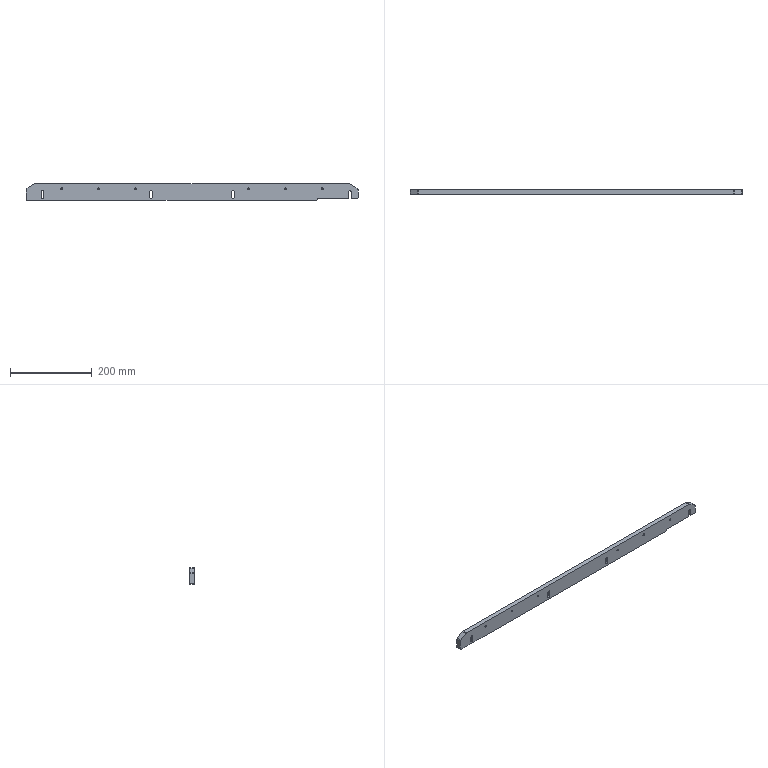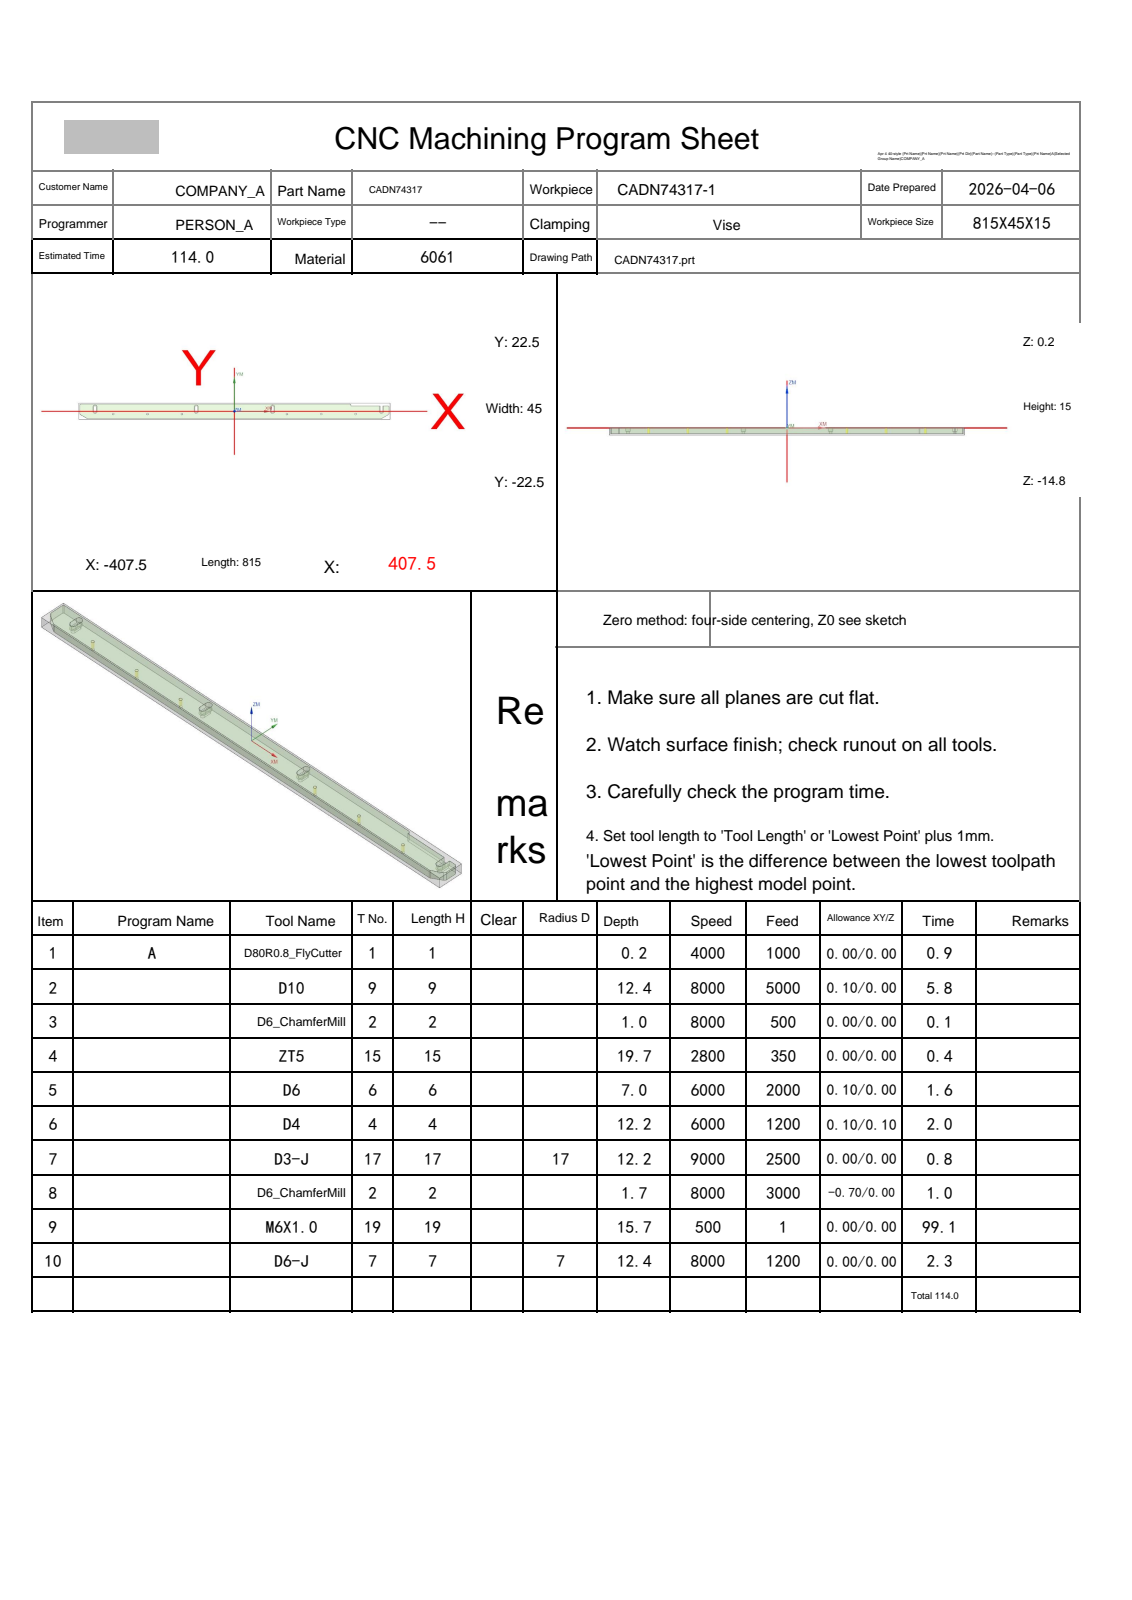NC program | NX | posted by the shop | part box 810 x 12 x 40 mm
Lines 1 to 1438 of 3610, first 1187 of 1436 lines:
%
O0001
(Machine time: 209.16 MIN)
(===Total Tool:9===)
(T1=D80R0.8 FlyCutter D=80.  R=0.8  D-  H01 Z=-0.   )
(T9=D10     D=10.  R=0.   D-  H09 Z=-12.2 )
(T2=D6_ChamferMill   D=6.   R=0.   D-  H02 Z=-1.5  )
(T15=ZT5    D=5.   DR_a=118 D-  H15 Z=-19.5 )
(T6=D6      D=6.   R=0.   D-  H06 Z=-6.8  )
(T4=D4      D=4.   R=0.   D-  H04 Z=-12.  )
(T17=D3-J   D=3.   R=0.   D17 H17 Z=-12.  )
(T19=M6X1.0 D=5.   DR_a=180 D-  H19 Z=-15.5 )
(T7=D6-J    D=6.   R=0.   D7  H07 Z=-12.2 )
G80 G90 G17 G49 G40
G91 G28 Z0
M01
N1 T01 M06
(D80R0.8 FlyCutter  D=80. R=0.8 H=01 ce=0.00 di=0.00)
G00 G90 G54 X450. Y0.0 M03 S4000
G43 H01 Z20.
M08
Z2.
G01 Z0.0 F1000.
X445.
X-445.
X-450.
Z2.
G00 Z20.
G91 G28 Z0.0
M05
M09
G91 G28 Z0.0
M01
N2 T09 M06
(D10  D=10. R=0. H=09 ce=0.10 di=0.00)
G00 G90 G54 X0.0 Y-25.1 M03 S8000
G43 H09 Z20.
M08
Z.5
G01 X-383.615 Z.322 F5000.
G02 X-388.811 Y-23.661 Z.319 I0.0 J10.1
G01 X-405.196 Y-13.83 Z.31
G02 X-410.1 Y-5.169 Z.306 I5.196 J8.661
G01 Y18. Z.295
G02 X-408.606 Y21.606 Z.293 I5.1 J0.0
G01 X-406.606 Y23.606 Z.292
G02 X-403. Y25.1 Z.29 I3.606 J-3.606
G01 X303. Z-.038
G02 X306.606 Y23.606 Z-.04 I0.0 J-5.1
G01 X308.606 Y21.606 Z-.041
G02 X309.648 Y20.1 Z-.042 I-3.606 J-3.606
G01 X381.7 Z-.076
G02 X385. Y18.888 Z-.077 I0.0 J-5.1
X388.3 Y20.1 Z-.079 I3.3 J-3.888
G01 X403. Z-.086
G02 X406.606 Y18.606 Z-.088 I0.0 J-5.1
G01 X408.606 Y16.606 Z-.089
G02 X410.1 Y13. Z-.091 I-3.606 J-3.606
G01 Y-5.169 Z-.099
G02 X405.196 Y-13.83 Z-.104 I-10.1 J0.0
G01 X388.811 Y-23.661 Z-.113
G02 X383.615 Y-25.1 Z-.116 I-5.196 J8.661
G01 X-383.615 Z-.472
G02 X-388.811 Y-23.661 Z-.474 I0.0 J10.1
G01 X-405.196 Y-13.83 Z-.483
G02 X-410.1 Y-5.169 Z-.488 I5.196 J8.661
G01 Y18. Z-.499
G02 X-408.606 Y21.606 Z-.501 I5.1 J0.0
G01 X-406.606 Y23.606 Z-.502
G02 X-403. Y25.1 Z-.504 I3.606 J-3.606
G01 X303. Z-.832
G02 X306.606 Y23.606 Z-.834 I0.0 J-5.1
G01 X308.606 Y21.606 Z-.835
G02 X309.648 Y20.1 Z-.836 I-3.606 J-3.606
G01 X381.7 Z-.869
G02 X385. Y18.888 Z-.871 I0.0 J-5.1
X388.3 Y20.1 Z-.873 I3.3 J-3.888
G01 X403. Z-.88
G02 X406.606 Y18.606 Z-.881 I0.0 J-5.1
G01 X408.606 Y16.606 Z-.883
G02 X410.1 Y13. Z-.885 I-3.606 J-3.606
G01 Y-5.169 Z-.893
G02 X405.196 Y-13.83 Z-.898 I-10.1 J0.0
G01 X388.811 Y-23.661 Z-.907
G02 X383.615 Y-25.1 Z-.909 I-5.196 J8.661
G01 X-383.615 Z-1.266
G02 X-388.811 Y-23.661 Z-1.268 I0.0 J10.1
G01 X-405.196 Y-13.83 Z-1.277
G02 X-410.1 Y-5.169 Z-1.282 I5.196 J8.661
G01 Y18. Z-1.293
G02 X-408.606 Y21.606 Z-1.295 I5.1 J0.0
G01 X-406.606 Y23.606 Z-1.296
G02 X-403. Y25.1 Z-1.298 I3.606 J-3.606
G01 X303. Z-1.626
G02 X306.606 Y23.606 Z-1.628 I0.0 J-5.1
G01 X308.606 Y21.606 Z-1.629
G02 X309.648 Y20.1 Z-1.63 I-3.606 J-3.606
G01 X381.7 Z-1.663
G02 X385. Y18.888 Z-1.665 I0.0 J-5.1
X388.3 Y20.1 Z-1.667 I3.3 J-3.888
G01 X403. Z-1.673
G02 X406.606 Y18.606 Z-1.675 I0.0 J-5.1
G01 X408.606 Y16.606 Z-1.677
G02 X410.1 Y13. Z-1.678 I-3.606 J-3.606
G01 Y-5.169 Z-1.687
G02 X405.196 Y-13.83 Z-1.692 I-10.1 J0.0
G01 X388.811 Y-23.661 Z-1.701
G02 X383.615 Y-25.1 Z-1.703 I-5.196 J8.661
G01 X-383.615 Z-2.059
G02 X-388.811 Y-23.661 Z-2.062 I0.0 J10.1
G01 X-405.196 Y-13.83 Z-2.071
G02 X-410.1 Y-5.169 Z-2.076 I5.196 J8.661
G01 Y18. Z-2.086
G02 X-408.606 Y21.606 Z-2.088 I5.1 J0.0
G01 X-406.606 Y23.606 Z-2.09
G02 X-403. Y25.1 Z-2.091 I3.606 J-3.606
G01 X303. Z-2.419
G02 X306.606 Y23.606 Z-2.421 I0.0 J-5.1
G01 X308.606 Y21.606 Z-2.423
G02 X309.648 Y20.1 Z-2.423 I-3.606 J-3.606
G01 X381.7 Z-2.457
G02 X385. Y18.888 Z-2.459 I0.0 J-5.1
X388.3 Y20.1 Z-2.46 I3.3 J-3.888
G01 X403. Z-2.467
G02 X406.606 Y18.606 Z-2.469 I0.0 J-5.1
G01 X408.606 Y16.606 Z-2.47
G02 X410.1 Y13. Z-2.472 I-3.606 J-3.606
G01 Y-5.169 Z-2.481
G02 X405.196 Y-13.83 Z-2.485 I-10.1 J0.0
G01 X388.811 Y-23.661 Z-2.494
G02 X383.615 Y-25.1 Z-2.497 I-5.196 J8.661
G01 X-383.615 Z-2.853
G02 X-388.811 Y-23.661 Z-2.856 I0.0 J10.1
G01 X-405.196 Y-13.83 Z-2.865
G02 X-410.1 Y-5.169 Z-2.869 I5.196 J8.661
G01 Y18. Z-2.88
G02 X-408.606 Y21.606 Z-2.882 I5.1 J0.0
G01 X-406.606 Y23.606 Z-2.883
G02 X-403. Y25.1 Z-2.885 I3.606 J-3.606
G01 X303. Z-3.213
G02 X306.606 Y23.606 Z-3.215 I0.0 J-5.1
G01 X308.606 Y21.606 Z-3.216
G02 X309.648 Y20.1 Z-3.217 I-3.606 J-3.606
G01 X381.7 Z-3.251
G02 X385. Y18.888 Z-3.252 I0.0 J-5.1
X388.3 Y20.1 Z-3.254 I3.3 J-3.888
G01 X403. Z-3.261
G02 X406.606 Y18.606 Z-3.263 I0.0 J-5.1
G01 X408.606 Y16.606 Z-3.264
G02 X410.1 Y13. Z-3.266 I-3.606 J-3.606
G01 Y-5.169 Z-3.274
G02 X405.196 Y-13.83 Z-3.279 I-10.1 J0.0
G01 X388.811 Y-23.661 Z-3.288
G02 X383.615 Y-25.1 Z-3.291 I-5.196 J8.661
G01 X-383.615 Z-3.647
G02 X-388.811 Y-23.661 Z-3.649 I0.0 J10.1
G01 X-405.196 Y-13.83 Z-3.658
G02 X-410.1 Y-5.169 Z-3.663 I5.196 J8.661
G01 Y18. Z-3.674
G02 X-408.606 Y21.606 Z-3.676 I5.1 J0.0
G01 X-406.606 Y23.606 Z-3.677
G02 X-403. Y25.1 Z-3.679 I3.606 J-3.606
G01 X303. Z-4.007
G02 X306.606 Y23.606 Z-4.009 I0.0 J-5.1
G01 X308.606 Y21.606 Z-4.01
G02 X309.648 Y20.1 Z-4.011 I-3.606 J-3.606
G01 X381.7 Z-4.044
G02 X385. Y18.888 Z-4.046 I0.0 J-5.1
X388.3 Y20.1 Z-4.048 I3.3 J-3.888
G01 X403. Z-4.055
G02 X406.606 Y18.606 Z-4.056 I0.0 J-5.1
G01 X408.606 Y16.606 Z-4.058
G02 X410.1 Y13. Z-4.06 I-3.606 J-3.606
G01 Y-5.169 Z-4.068
G02 X405.196 Y-13.83 Z-4.073 I-10.1 J0.0
G01 X388.811 Y-23.661 Z-4.082
G02 X383.615 Y-25.1 Z-4.084 I-5.196 J8.661
G01 X-383.615 Z-4.441
G02 X-388.811 Y-23.661 Z-4.443 I0.0 J10.1
G01 X-405.196 Y-13.83 Z-4.452
G02 X-410.1 Y-5.169 Z-4.457 I5.196 J8.661
G01 Y18. Z-4.468
G02 X-408.606 Y21.606 Z-4.47 I5.1 J0.0
G01 X-406.606 Y23.606 Z-4.471
G02 X-403. Y25.1 Z-4.473 I3.606 J-3.606
G01 X303. Z-4.801
G02 X306.606 Y23.606 Z-4.803 I0.0 J-5.1
G01 X308.606 Y21.606 Z-4.804
G02 X309.648 Y20.1 Z-4.805 I-3.606 J-3.606
G01 X381.7 Z-4.838
G02 X385. Y18.888 Z-4.84 I0.0 J-5.1
X388.3 Y20.1 Z-4.842 I3.3 J-3.888
G01 X403. Z-4.848
G02 X406.606 Y18.606 Z-4.85 I0.0 J-5.1
G01 X408.606 Y16.606 Z-4.852
G02 X410.1 Y13. Z-4.853 I-3.606 J-3.606
G01 Y-5.169 Z-4.862
G02 X405.196 Y-13.83 Z-4.867 I-10.1 J0.0
G01 X388.811 Y-23.661 Z-4.876
G02 X383.615 Y-25.1 Z-4.878 I-5.196 J8.661
G01 X-383.615 Z-5.234
G02 X-388.811 Y-23.661 Z-5.237 I0.0 J10.1
G01 X-405.196 Y-13.83 Z-5.246
G02 X-410.1 Y-5.169 Z-5.251 I5.196 J8.661
G01 Y18. Z-5.261
G02 X-408.606 Y21.606 Z-5.263 I5.1 J0.0
G01 X-406.606 Y23.606 Z-5.265
G02 X-403. Y25.1 Z-5.266 I3.606 J-3.606
G01 X303. Z-5.594
G02 X306.606 Y23.606 Z-5.596 I0.0 J-5.1
G01 X308.606 Y21.606 Z-5.598
G02 X309.648 Y20.1 Z-5.598 I-3.606 J-3.606
G01 X381.7 Z-5.632
G02 X385. Y18.888 Z-5.634 I0.0 J-5.1
X388.3 Y20.1 Z-5.635 I3.3 J-3.888
G01 X403. Z-5.642
G02 X406.606 Y18.606 Z-5.644 I0.0 J-5.1
G01 X408.606 Y16.606 Z-5.645
G02 X410.1 Y13. Z-5.647 I-3.606 J-3.606
G01 Y-5.169 Z-5.656
G02 X405.196 Y-13.83 Z-5.66 I-10.1 J0.0
G01 X388.811 Y-23.661 Z-5.669
G02 X383.615 Y-25.1 Z-5.672 I-5.196 J8.661
G01 X-383.615 Z-6.028
G02 X-388.811 Y-23.661 Z-6.031 I0.0 J10.1
G01 X-405.196 Y-13.83 Z-6.04
G02 X-410.1 Y-5.169 Z-6.044 I5.196 J8.661
G01 Y18. Z-6.055
G02 X-408.606 Y21.606 Z-6.057 I5.1 J0.0
G01 X-406.606 Y23.606 Z-6.058
G02 X-403. Y25.1 Z-6.06 I3.606 J-3.606
G01 X303. Z-6.388
G02 X306.606 Y23.606 Z-6.39 I0.0 J-5.1
G01 X308.606 Y21.606 Z-6.391
G02 X309.648 Y20.1 Z-6.392 I-3.606 J-3.606
G01 X381.7 Z-6.426
G02 X385. Y18.888 Z-6.427 I0.0 J-5.1
X388.3 Y20.1 Z-6.429 I3.3 J-3.888
G01 X403. Z-6.436
G02 X406.606 Y18.606 Z-6.438 I0.0 J-5.1
G01 X408.606 Y16.606 Z-6.439
G02 X410.1 Y13. Z-6.441 I-3.606 J-3.606
G01 Y-5.169 Z-6.449
G02 X405.196 Y-13.83 Z-6.454 I-10.1 J0.0
G01 X388.811 Y-23.661 Z-6.463
G02 X383.615 Y-25.1 Z-6.466 I-5.196 J8.661
G01 X-383.615 Z-6.822
G02 X-388.811 Y-23.661 Z-6.824 I0.0 J10.1
G01 X-405.196 Y-13.83 Z-6.833
G02 X-410.1 Y-5.169 Z-6.838 I5.196 J8.661
G01 Y18. Z-6.849
G02 X-408.606 Y21.606 Z-6.851 I5.1 J0.0
G01 X-406.606 Y23.606 Z-6.852
G02 X-403. Y25.1 Z-6.854 I3.606 J-3.606
G01 X303. Z-7.182
G02 X306.606 Y23.606 Z-7.184 I0.0 J-5.1
G01 X308.606 Y21.606 Z-7.185
G02 X309.648 Y20.1 Z-7.186 I-3.606 J-3.606
G01 X381.7 Z-7.219
G02 X385. Y18.888 Z-7.221 I0.0 J-5.1
X388.3 Y20.1 Z-7.223 I3.3 J-3.888
G01 X403. Z-7.23
G02 X406.606 Y18.606 Z-7.231 I0.0 J-5.1
G01 X408.606 Y16.606 Z-7.233
G02 X410.1 Y13. Z-7.235 I-3.606 J-3.606
G01 Y-5.169 Z-7.243
G02 X405.196 Y-13.83 Z-7.248 I-10.1 J0.0
G01 X388.811 Y-23.661 Z-7.257
G02 X383.615 Y-25.1 Z-7.259 I-5.196 J8.661
G01 X-383.615 Z-7.616
G02 X-388.811 Y-23.661 Z-7.618 I0.0 J10.1
G01 X-405.196 Y-13.83 Z-7.627
G02 X-410.1 Y-5.169 Z-7.632 I5.196 J8.661
G01 Y18. Z-7.643
G02 X-408.606 Y21.606 Z-7.645 I5.1 J0.0
G01 X-406.606 Y23.606 Z-7.646
G02 X-403. Y25.1 Z-7.648 I3.606 J-3.606
G01 X303. Z-7.976
G02 X306.606 Y23.606 Z-7.978 I0.0 J-5.1
G01 X308.606 Y21.606 Z-7.979
G02 X309.648 Y20.1 Z-7.98 I-3.606 J-3.606
G01 X381.7 Z-8.013
G02 X385. Y18.888 Z-8.015 I0.0 J-5.1
X388.3 Y20.1 Z-8.017 I3.3 J-3.888
G01 X403. Z-8.023
G02 X406.606 Y18.606 Z-8.025 I0.0 J-5.1
G01 X408.606 Y16.606 Z-8.027
G02 X410.1 Y13. Z-8.028 I-3.606 J-3.606
G01 Y-5.169 Z-8.037
G02 X405.196 Y-13.83 Z-8.042 I-10.1 J0.0
G01 X388.811 Y-23.661 Z-8.051
G02 X383.615 Y-25.1 Z-8.053 I-5.196 J8.661
G01 X-383.615 Z-8.409
G02 X-388.811 Y-23.661 Z-8.412 I0.0 J10.1
G01 X-405.196 Y-13.83 Z-8.421
G02 X-410.1 Y-5.169 Z-8.426 I5.196 J8.661
G01 Y18. Z-8.436
G02 X-408.606 Y21.606 Z-8.438 I5.1 J0.0
G01 X-406.606 Y23.606 Z-8.44
G02 X-403. Y25.1 Z-8.441 I3.606 J-3.606
G01 X303. Z-8.769
G02 X306.606 Y23.606 Z-8.771 I0.0 J-5.1
G01 X308.606 Y21.606 Z-8.773
G02 X309.648 Y20.1 Z-8.773 I-3.606 J-3.606
G01 X381.7 Z-8.807
G02 X385. Y18.888 Z-8.809 I0.0 J-5.1
X388.3 Y20.1 Z-8.81 I3.3 J-3.888
G01 X403. Z-8.817
G02 X406.606 Y18.606 Z-8.819 I0.0 J-5.1
G01 X408.606 Y16.606 Z-8.82
G02 X410.1 Y13. Z-8.822 I-3.606 J-3.606
G01 Y-5.169 Z-8.831
G02 X405.196 Y-13.83 Z-8.835 I-10.1 J0.0
G01 X388.811 Y-23.661 Z-8.844
G02 X383.615 Y-25.1 Z-8.847 I-5.196 J8.661
G01 X-383.615 Z-9.203
G02 X-388.811 Y-23.661 Z-9.206 I0.0 J10.1
G01 X-405.196 Y-13.83 Z-9.215
G02 X-410.1 Y-5.169 Z-9.219 I5.196 J8.661
G01 Y18. Z-9.23
G02 X-408.606 Y21.606 Z-9.232 I5.1 J0.0
G01 X-406.606 Y23.606 Z-9.233
G02 X-403. Y25.1 Z-9.235 I3.606 J-3.606
G01 X303. Z-9.563
G02 X306.606 Y23.606 Z-9.565 I0.0 J-5.1
G01 X308.606 Y21.606 Z-9.566
G02 X309.648 Y20.1 Z-9.567 I-3.606 J-3.606
G01 X381.7 Z-9.601
G02 X385. Y18.888 Z-9.602 I0.0 J-5.1
X388.3 Y20.1 Z-9.604 I3.3 J-3.888
G01 X403. Z-9.611
G02 X406.606 Y18.606 Z-9.613 I0.0 J-5.1
G01 X408.606 Y16.606 Z-9.614
G02 X410.1 Y13. Z-9.616 I-3.606 J-3.606
G01 Y-5.169 Z-9.624
G02 X405.196 Y-13.83 Z-9.629 I-10.1 J0.0
G01 X388.811 Y-23.661 Z-9.638
G02 X383.615 Y-25.1 Z-9.641 I-5.196 J8.661
G01 X-383.615 Z-9.997
G02 X-388.811 Y-23.661 Z-9.999 I0.0 J10.1
G01 X-405.196 Y-13.83 Z-10.008
G02 X-410.1 Y-5.169 Z-10.013 I5.196 J8.661
G01 Y18. Z-10.024
G02 X-408.606 Y21.606 Z-10.026 I5.1 J0.0
G01 X-406.606 Y23.606 Z-10.027
G02 X-403. Y25.1 Z-10.029 I3.606 J-3.606
G01 X303. Z-10.357
G02 X306.606 Y23.606 Z-10.359 I0.0 J-5.1
G01 X308.606 Y21.606 Z-10.36
G02 X309.648 Y20.1 Z-10.361 I-3.606 J-3.606
G01 X381.7 Z-10.394
G02 X385. Y18.888 Z-10.396 I0.0 J-5.1
X388.3 Y20.1 Z-10.398 I3.3 J-3.888
G01 X403. Z-10.405
G02 X406.606 Y18.606 Z-10.406 I0.0 J-5.1
G01 X408.606 Y16.606 Z-10.408
G02 X410.1 Y13. Z-10.41 I-3.606 J-3.606
G01 Y-5.169 Z-10.418
G02 X405.196 Y-13.83 Z-10.423 I-10.1 J0.0
G01 X388.811 Y-23.661 Z-10.432
G02 X383.615 Y-25.1 Z-10.434 I-5.196 J8.661
G01 X-383.615 Z-10.791
G02 X-388.811 Y-23.661 Z-10.793 I0.0 J10.1
G01 X-405.196 Y-13.83 Z-10.802
G02 X-410.1 Y-5.169 Z-10.807 I5.196 J8.661
G01 Y18. Z-10.818
G02 X-408.606 Y21.606 Z-10.82 I5.1 J0.0
G01 X-406.606 Y23.606 Z-10.821
G02 X-403. Y25.1 Z-10.823 I3.606 J-3.606
G01 X303. Z-11.151
G02 X306.606 Y23.606 Z-11.153 I0.0 J-5.1
G01 X308.606 Y21.606 Z-11.154
G02 X309.648 Y20.1 Z-11.155 I-3.606 J-3.606
G01 X381.7 Z-11.188
G02 X385. Y18.888 Z-11.19 I0.0 J-5.1
X388.3 Y20.1 Z-11.192 I3.3 J-3.888
G01 X403. Z-11.198
G02 X406.606 Y18.606 Z-11.2 I0.0 J-5.1
G01 X408.606 Y16.606 Z-11.202
G02 X410.1 Y13. Z-11.203 I-3.606 J-3.606
G01 Y-5.169 Z-11.212
G02 X405.196 Y-13.83 Z-11.217 I-10.1 J0.0
G01 X388.811 Y-23.661 Z-11.226
G02 X383.615 Y-25.1 Z-11.228 I-5.196 J8.661
G01 X-383.615 Z-11.584
G02 X-388.811 Y-23.661 Z-11.587 I0.0 J10.1
G01 X-405.196 Y-13.83 Z-11.596
G02 X-410.1 Y-5.169 Z-11.601 I5.196 J8.661
G01 Y18. Z-11.611
G02 X-408.606 Y21.606 Z-11.613 I5.1 J0.0
G01 X-406.606 Y23.606 Z-11.615
G02 X-403. Y25.1 Z-11.616 I3.606 J-3.606
G01 X303. Z-11.944
G02 X306.606 Y23.606 Z-11.946 I0.0 J-5.1
G01 X308.606 Y21.606 Z-11.948
G02 X309.648 Y20.1 Z-11.948 I-3.606 J-3.606
G01 X381.7 Z-11.982
G02 X385. Y18.888 Z-11.984 I0.0 J-5.1
X388.3 Y20.1 Z-11.985 I3.3 J-3.888
G01 X403. Z-11.992
G02 X406.606 Y18.606 Z-11.994 I0.0 J-5.1
G01 X408.606 Y16.606 Z-11.995
G02 X410.1 Y13. Z-11.997 I-3.606 J-3.606
G01 Y-5.169 Z-12.006
G02 X405.196 Y-13.83 Z-12.01 I-10.1 J0.0
G01 X388.811 Y-23.661 Z-12.019
G02 X383.615 Y-25.1 Z-12.022 I-5.196 J8.661
G01 X0.0 Z-12.2
X-383.615
G02 X-388.811 Y-23.661 I0.0 J10.1
G01 X-405.196 Y-13.83
G02 X-410.1 Y-5.169 I5.196 J8.661
G01 Y18.
G02 X-408.606 Y21.606 I5.1 J0.0
G01 X-406.606 Y23.606
G02 X-403. Y25.1 I3.606 J-3.606
G01 X303.
G02 X306.606 Y23.606 I0.0 J-5.1
G01 X308.606 Y21.606
G02 X309.648 Y20.1 I-3.606 J-3.606
G01 X381.7
G02 X385. Y18.888 I0.0 J-5.1
X388.3 Y20.1 I3.3 J-3.888
G01 X403.
G02 X406.606 Y18.606 I0.0 J-5.1
G01 X408.606 Y16.606
G02 X410.1 Y13. I-3.606 J-3.606
G01 Y-5.169
G02 X405.196 Y-13.83 I-10.1 J0.0
G01 X388.811 Y-23.661
G02 X383.615 Y-25.1 I-5.196 J8.661
G01 X0.0
X-.5
Z-11.2
G00 Z20.
G91 G28 Z0.0
M05
M09
G91 G28 Z0.0
M01
N3 T02 M06
(D6_ChamferMill  D=6. R=0. H=02 ce=0.00 di=0.00)
G00 G90 G54 X-317.5 Y-7.5 M03 S8000
G43 H02 Z20.
M08
G98 G81 X-317.5 Y-7.5 Z-.8 R1. F500.
X-227.5
X-137.5
X137.5
X227.5
X317.5
G80
G00 Z20.
G91 G28 Z0.0
M05
M09
G91 G28 Z0.0
M01
N4 T15 M06
(ZT5 D=5. DR_a=118 H=15)
G00 G90 G54 X-317.5 Y-7.5 M03 S2800
G43 H15 Z20.
M08
G98 G83 X-317.5 Y-7.5 Z-19.502 R1. F350. Q3.
X-227.5
X-137.5
X137.5
X227.5
X317.5
G80
G00 Z20.
G91 G28 Z0.0
M05
M09
G91 G28 Z0.0
M01
N5 T06 M06
(D6  D=6. R=0. H=06 ce=0.10 di=0.00)
G00 G90 G54 X-362.6 Y6. M03 S6000
G43 H06 Z20.
M08
Z.5
G01 Y12. Z.455 F2000.
G03 X-365. Y14.4 Z.427 I-2.4 J0.0
X-367.4 Y12. Z.399 I0.0 J-2.4
G01 Y0.0 Z.309
G03 X-365. Y-2.4 Z.281 I2.4 J0.0
X-362.6 Y0.0 Z.253 I0.0 J2.4
G01 Y12. Z.163
G03 X-365. Y14.4 Z.135 I-2.4 J0.0
X-367.4 Y12. Z.107 I0.0 J-2.4
G01 Y0.0 Z.017
G03 X-365. Y-2.4 Z-.011 I2.4 J0.0
X-362.6 Y0.0 Z-.039 I0.0 J2.4
G01 Y12. Z-.129
G03 X-365. Y14.4 Z-.157 I-2.4 J0.0
X-367.4 Y12. Z-.185 I0.0 J-2.4
G01 Y0.0 Z-.275
G03 X-365. Y-2.4 Z-.303 I2.4 J0.0
X-362.6 Y0.0 Z-.331 I0.0 J2.4
G01 Y12. Z-.421
G03 X-365. Y14.4 Z-.449 I-2.4 J0.0
X-367.4 Y12. Z-.477 I0.0 J-2.4
G01 Y0.0 Z-.567
G03 X-365. Y-2.4 Z-.595 I2.4 J0.0
X-362.6 Y0.0 Z-.623 I0.0 J2.4
G01 Y12. Z-.713
G03 X-365. Y14.4 Z-.741 I-2.4 J0.0
X-367.4 Y12. Z-.769 I0.0 J-2.4
G01 Y0.0 Z-.859
G03 X-365. Y-2.4 Z-.887 I2.4 J0.0
X-362.6 Y0.0 Z-.915 I0.0 J2.4
G01 Y12. Z-1.005
G03 X-365. Y14.4 Z-1.033 I-2.4 J0.0
X-367.4 Y12. Z-1.061 I0.0 J-2.4
G01 Y0.0 Z-1.151
G03 X-365. Y-2.4 Z-1.179 I2.4 J0.0
X-362.6 Y0.0 Z-1.207 I0.0 J2.4
G01 Y12. Z-1.297
G03 X-365. Y14.4 Z-1.325 I-2.4 J0.0
X-367.4 Y12. Z-1.353 I0.0 J-2.4
G01 Y0.0 Z-1.443
G03 X-365. Y-2.4 Z-1.471 I2.4 J0.0
X-362.6 Y0.0 Z-1.499 I0.0 J2.4
G01 Y12. Z-1.589
G03 X-365. Y14.4 Z-1.617 I-2.4 J0.0
X-367.4 Y12. Z-1.645 I0.0 J-2.4
G01 Y0.0 Z-1.735
G03 X-365. Y-2.4 Z-1.763 I2.4 J0.0
X-362.6 Y0.0 Z-1.791 I0.0 J2.4
G01 Y12. Z-1.881
G03 X-365. Y14.4 Z-1.909 I-2.4 J0.0
X-367.4 Y12. Z-1.937 I0.0 J-2.4
G01 Y0.0 Z-2.027
G03 X-365. Y-2.4 Z-2.055 I2.4 J0.0
X-362.6 Y0.0 Z-2.083 I0.0 J2.4
G01 Y12. Z-2.173
G03 X-365. Y14.4 Z-2.201 I-2.4 J0.0
X-367.4 Y12. Z-2.229 I0.0 J-2.4
G01 Y0.0 Z-2.319
G03 X-365. Y-2.4 Z-2.347 I2.4 J0.0
X-362.6 Y0.0 Z-2.375 I0.0 J2.4
G01 Y12. Z-2.465
G03 X-365. Y14.4 Z-2.493 I-2.4 J0.0
X-367.4 Y12. Z-2.521 I0.0 J-2.4
G01 Y0.0 Z-2.611
G03 X-365. Y-2.4 Z-2.639 I2.4 J0.0
X-362.6 Y0.0 Z-2.667 I0.0 J2.4
G01 Y12. Z-2.757
G03 X-365. Y14.4 Z-2.785 I-2.4 J0.0
X-367.4 Y12. Z-2.813 I0.0 J-2.4
G01 Y0.0 Z-2.903
G03 X-365. Y-2.4 Z-2.931 I2.4 J0.0
X-362.6 Y0.0 Z-2.959 I0.0 J2.4
G01 Y12. Z-3.049
G03 X-365. Y14.4 Z-3.077 I-2.4 J0.0
X-367.4 Y12. Z-3.105 I0.0 J-2.4
G01 Y0.0 Z-3.195
G03 X-365. Y-2.4 Z-3.223 I2.4 J0.0
X-362.6 Y0.0 Z-3.251 I0.0 J2.4
G01 Y12. Z-3.341
G03 X-365. Y14.4 Z-3.369 I-2.4 J0.0
X-367.4 Y12. Z-3.397 I0.0 J-2.4
G01 Y0.0 Z-3.487
G03 X-365. Y-2.4 Z-3.515 I2.4 J0.0
X-362.6 Y0.0 Z-3.543 I0.0 J2.4
G01 Y12. Z-3.633
G03 X-365. Y14.4 Z-3.661 I-2.4 J0.0
X-367.4 Y12. Z-3.689 I0.0 J-2.4
G01 Y0.0 Z-3.779
G03 X-365. Y-2.4 Z-3.807 I2.4 J0.0
X-362.6 Y0.0 Z-3.835 I0.0 J2.4
G01 Y12. Z-3.925
G03 X-365. Y14.4 Z-3.953 I-2.4 J0.0
X-367.4 Y12. Z-3.981 I0.0 J-2.4
G01 Y0.0 Z-4.071
G03 X-365. Y-2.4 Z-4.099 I2.4 J0.0
X-362.6 Y0.0 Z-4.127 I0.0 J2.4
G01 Y12. Z-4.217
G03 X-365. Y14.4 Z-4.245 I-2.4 J0.0
X-367.4 Y12. Z-4.273 I0.0 J-2.4
G01 Y0.0 Z-4.363
G03 X-365. Y-2.4 Z-4.391 I2.4 J0.0
X-362.6 Y0.0 Z-4.419 I0.0 J2.4
G01 Y12. Z-4.509
G03 X-365. Y14.4 Z-4.537 I-2.4 J0.0
X-367.4 Y12. Z-4.565 I0.0 J-2.4
G01 Y0.0 Z-4.655
G03 X-365. Y-2.4 Z-4.683 I2.4 J0.0
X-362.6 Y0.0 Z-4.711 I0.0 J2.4
G01 Y12. Z-4.801
G03 X-365. Y14.4 Z-4.829 I-2.4 J0.0
X-367.4 Y12. Z-4.857 I0.0 J-2.4
G01 Y0.0 Z-4.947
G03 X-365. Y-2.4 Z-4.975 I2.4 J0.0
X-362.6 Y0.0 Z-5.003 I0.0 J2.4
G01 Y12. Z-5.093
G03 X-365. Y14.4 Z-5.121 I-2.4 J0.0
X-367.4 Y12. Z-5.149 I0.0 J-2.4
G01 Y0.0 Z-5.239
G03 X-365. Y-2.4 Z-5.267 I2.4 J0.0
X-362.6 Y0.0 Z-5.295 I0.0 J2.4
G01 Y12. Z-5.385
G03 X-365. Y14.4 Z-5.413 I-2.4 J0.0
X-367.4 Y12. Z-5.441 I0.0 J-2.4
G01 Y0.0 Z-5.531
G03 X-365. Y-2.4 Z-5.559 I2.4 J0.0
X-362.6 Y0.0 Z-5.587 I0.0 J2.4
G01 Y12. Z-5.677
G03 X-365. Y14.4 Z-5.705 I-2.4 J0.0
X-367.4 Y12. Z-5.733 I0.0 J-2.4
G01 Y0.0 Z-5.823
G03 X-365. Y-2.4 Z-5.851 I2.4 J0.0
X-362.6 Y0.0 Z-5.879 I0.0 J2.4
G01 Y12. Z-5.969
G03 X-365. Y14.4 Z-5.997 I-2.4 J0.0
X-367.4 Y12. Z-6.025 I0.0 J-2.4
G01 Y0.0 Z-6.115
G03 X-365. Y-2.4 Z-6.143 I2.4 J0.0
X-362.6 Y0.0 Z-6.171 I0.0 J2.4
G01 Y12. Z-6.261
G03 X-365. Y14.4 Z-6.289 I-2.4 J0.0
X-367.4 Y12. Z-6.317 I0.0 J-2.4
G01 Y0.0 Z-6.407
G03 X-365. Y-2.4 Z-6.435 I2.4 J0.0
X-362.6 Y0.0 Z-6.463 I0.0 J2.4
G01 Y12. Z-6.553
G03 X-365. Y14.4 Z-6.581 I-2.4 J0.0
X-367.4 Y12. Z-6.609 I0.0 J-2.4
G01 Y0.0 Z-6.699
G03 X-365. Y-2.4 Z-6.727 I2.4 J0.0
X-362.6 Y0.0 Z-6.755 I0.0 J2.4
G01 Y6. Z-6.8
Y12.
G03 X-365. Y14.4 I-2.4 J0.0
X-367.4 Y12. I0.0 J-2.4
G01 Y0.0
G03 X-365. Y-2.4 I2.4 J0.0
X-362.6 Y0.0 I0.0 J2.4
G01 Y6.
Y6.5
Z-5.8
G00 Z20.
X-102.4 Y6.
Z.5
G01 Y0.0 Z.455
G03 X-100. Y-2.4 Z.427 I2.4 J0.0
X-97.6 Y0.0 Z.399 I0.0 J2.4
G01 Y12. Z.309
G03 X-100. Y14.4 Z.281 I-2.4 J0.0
X-102.4 Y12. Z.253 I0.0 J-2.4
G01 Y0.0 Z.163
G03 X-100. Y-2.4 Z.135 I2.4 J0.0
X-97.6 Y0.0 Z.107 I0.0 J2.4
G01 Y12. Z.017
G03 X-100. Y14.4 Z-.011 I-2.4 J0.0
X-102.4 Y12. Z-.039 I0.0 J-2.4
G01 Y0.0 Z-.129
G03 X-100. Y-2.4 Z-.157 I2.4 J0.0
X-97.6 Y0.0 Z-.185 I0.0 J2.4
G01 Y12. Z-.275
G03 X-100. Y14.4 Z-.303 I-2.4 J0.0
X-102.4 Y12. Z-.331 I0.0 J-2.4
G01 Y0.0 Z-.421
G03 X-100. Y-2.4 Z-.449 I2.4 J0.0
X-97.6 Y0.0 Z-.477 I0.0 J2.4
G01 Y12. Z-.567
G03 X-100. Y14.4 Z-.595 I-2.4 J0.0
X-102.4 Y12. Z-.623 I0.0 J-2.4
G01 Y0.0 Z-.713
G03 X-100. Y-2.4 Z-.741 I2.4 J0.0
X-97.6 Y0.0 Z-.769 I0.0 J2.4
G01 Y12. Z-.859
G03 X-100. Y14.4 Z-.887 I-2.4 J0.0
X-102.4 Y12. Z-.915 I0.0 J-2.4
G01 Y0.0 Z-1.005
G03 X-100. Y-2.4 Z-1.033 I2.4 J0.0
X-97.6 Y0.0 Z-1.061 I0.0 J2.4
G01 Y12. Z-1.151
G03 X-100. Y14.4 Z-1.179 I-2.4 J0.0
X-102.4 Y12. Z-1.207 I0.0 J-2.4
G01 Y0.0 Z-1.297
G03 X-100. Y-2.4 Z-1.325 I2.4 J0.0
X-97.6 Y0.0 Z-1.353 I0.0 J2.4
G01 Y12. Z-1.443
G03 X-100. Y14.4 Z-1.471 I-2.4 J0.0
X-102.4 Y12. Z-1.499 I0.0 J-2.4
G01 Y0.0 Z-1.589
G03 X-100. Y-2.4 Z-1.617 I2.4 J0.0
X-97.6 Y0.0 Z-1.645 I0.0 J2.4
G01 Y12. Z-1.735
G03 X-100. Y14.4 Z-1.763 I-2.4 J0.0
X-102.4 Y12. Z-1.791 I0.0 J-2.4
G01 Y0.0 Z-1.881
G03 X-100. Y-2.4 Z-1.909 I2.4 J0.0
X-97.6 Y0.0 Z-1.937 I0.0 J2.4
G01 Y12. Z-2.027
G03 X-100. Y14.4 Z-2.055 I-2.4 J0.0
X-102.4 Y12. Z-2.083 I0.0 J-2.4
G01 Y0.0 Z-2.173
G03 X-100. Y-2.4 Z-2.201 I2.4 J0.0
X-97.6 Y0.0 Z-2.229 I0.0 J2.4
G01 Y12. Z-2.319
G03 X-100. Y14.4 Z-2.347 I-2.4 J0.0
X-102.4 Y12. Z-2.375 I0.0 J-2.4
G01 Y0.0 Z-2.465
G03 X-100. Y-2.4 Z-2.493 I2.4 J0.0
X-97.6 Y0.0 Z-2.521 I0.0 J2.4
G01 Y12. Z-2.611
G03 X-100. Y14.4 Z-2.639 I-2.4 J0.0
X-102.4 Y12. Z-2.667 I0.0 J-2.4
G01 Y0.0 Z-2.757
G03 X-100. Y-2.4 Z-2.785 I2.4 J0.0
X-97.6 Y0.0 Z-2.813 I0.0 J2.4
G01 Y12. Z-2.903
G03 X-100. Y14.4 Z-2.931 I-2.4 J0.0
X-102.4 Y12. Z-2.959 I0.0 J-2.4
G01 Y0.0 Z-3.049
G03 X-100. Y-2.4 Z-3.077 I2.4 J0.0
X-97.6 Y0.0 Z-3.105 I0.0 J2.4
G01 Y12. Z-3.195
G03 X-100. Y14.4 Z-3.223 I-2.4 J0.0
X-102.4 Y12. Z-3.251 I0.0 J-2.4
G01 Y0.0 Z-3.341
G03 X-100. Y-2.4 Z-3.369 I2.4 J0.0
X-97.6 Y0.0 Z-3.397 I0.0 J2.4
G01 Y12. Z-3.487
G03 X-100. Y14.4 Z-3.515 I-2.4 J0.0
X-102.4 Y12. Z-3.543 I0.0 J-2.4
G01 Y0.0 Z-3.633
G03 X-100. Y-2.4 Z-3.661 I2.4 J0.0
X-97.6 Y0.0 Z-3.689 I0.0 J2.4
G01 Y12. Z-3.779
G03 X-100. Y14.4 Z-3.807 I-2.4 J0.0
X-102.4 Y12. Z-3.835 I0.0 J-2.4
G01 Y0.0 Z-3.925
G03 X-100. Y-2.4 Z-3.953 I2.4 J0.0
X-97.6 Y0.0 Z-3.981 I0.0 J2.4
G01 Y12. Z-4.071
G03 X-100. Y14.4 Z-4.099 I-2.4 J0.0
X-102.4 Y12. Z-4.127 I0.0 J-2.4
G01 Y0.0 Z-4.217
G03 X-100. Y-2.4 Z-4.245 I2.4 J0.0
X-97.6 Y0.0 Z-4.273 I0.0 J2.4
G01 Y12. Z-4.363
G03 X-100. Y14.4 Z-4.391 I-2.4 J0.0
X-102.4 Y12. Z-4.419 I0.0 J-2.4
G01 Y0.0 Z-4.509
G03 X-100. Y-2.4 Z-4.537 I2.4 J0.0
X-97.6 Y0.0 Z-4.565 I0.0 J2.4
G01 Y12. Z-4.655
G03 X-100. Y14.4 Z-4.683 I-2.4 J0.0
X-102.4 Y12. Z-4.711 I0.0 J-2.4
G01 Y0.0 Z-4.801
G03 X-100. Y-2.4 Z-4.829 I2.4 J0.0
X-97.6 Y0.0 Z-4.857 I0.0 J2.4
G01 Y12. Z-4.947
G03 X-100. Y14.4 Z-4.975 I-2.4 J0.0
X-102.4 Y12. Z-5.003 I0.0 J-2.4
G01 Y0.0 Z-5.093
G03 X-100. Y-2.4 Z-5.121 I2.4 J0.0
X-97.6 Y0.0 Z-5.149 I0.0 J2.4
G01 Y12. Z-5.239
G03 X-100. Y14.4 Z-5.267 I-2.4 J0.0
X-102.4 Y12. Z-5.295 I0.0 J-2.4
G01 Y0.0 Z-5.385
G03 X-100. Y-2.4 Z-5.413 I2.4 J0.0
X-97.6 Y0.0 Z-5.441 I0.0 J2.4
G01 Y12. Z-5.531
G03 X-100. Y14.4 Z-5.559 I-2.4 J0.0
X-102.4 Y12. Z-5.587 I0.0 J-2.4
G01 Y0.0 Z-5.677
G03 X-100. Y-2.4 Z-5.705 I2.4 J0.0
X-97.6 Y0.0 Z-5.733 I0.0 J2.4
G01 Y12. Z-5.823
G03 X-100. Y14.4 Z-5.851 I-2.4 J0.0
X-102.4 Y12. Z-5.879 I0.0 J-2.4
G01 Y0.0 Z-5.969
G03 X-100. Y-2.4 Z-5.997 I2.4 J0.0
X-97.6 Y0.0 Z-6.025 I0.0 J2.4
G01 Y12. Z-6.115
G03 X-100. Y14.4 Z-6.143 I-2.4 J0.0
X-102.4 Y12. Z-6.171 I0.0 J-2.4
G01 Y0.0 Z-6.261
G03 X-100. Y-2.4 Z-6.289 I2.4 J0.0
X-97.6 Y0.0 Z-6.317 I0.0 J2.4
G01 Y12. Z-6.407
G03 X-100. Y14.4 Z-6.435 I-2.4 J0.0
X-102.4 Y12. Z-6.463 I0.0 J-2.4
G01 Y0.0 Z-6.553
G03 X-100. Y-2.4 Z-6.581 I2.4 J0.0
X-97.6 Y0.0 Z-6.609 I0.0 J2.4
G01 Y12. Z-6.699
G03 X-100. Y14.4 Z-6.727 I-2.4 J0.0
X-102.4 Y12. Z-6.755 I0.0 J-2.4
G01 Y6. Z-6.8
Y0.0
G03 X-100. Y-2.4 I2.4 J0.0
X-97.6 Y0.0 I0.0 J2.4
G01 Y12.
G03 X-100. Y14.4 I-2.4 J0.0
X-102.4 Y12. I0.0 J-2.4
G01 Y6.
Y5.5
Z-5.8
G00 Z20.
X97.6 Y6.
Z.5
G01 Y0.0 Z.455
G03 X100. Y-2.4 Z.427 I2.4 J0.0
X102.4 Y0.0 Z.399 I0.0 J2.4
G01 Y12. Z.309
G03 X100. Y14.4 Z.281 I-2.4 J0.0
X97.6 Y12. Z.253 I0.0 J-2.4
G01 Y0.0 Z.163
G03 X100. Y-2.4 Z.135 I2.4 J0.0
X102.4 Y0.0 Z.107 I0.0 J2.4
G01 Y12. Z.017
G03 X100. Y14.4 Z-.011 I-2.4 J0.0
X97.6 Y12. Z-.039 I0.0 J-2.4
G01 Y0.0 Z-.129
G03 X100. Y-2.4 Z-.157 I2.4 J0.0
X102.4 Y0.0 Z-.185 I0.0 J2.4
G01 Y12. Z-.275
G03 X100. Y14.4 Z-.303 I-2.4 J0.0
X97.6 Y12. Z-.331 I0.0 J-2.4
G01 Y0.0 Z-.421
G03 X100. Y-2.4 Z-.449 I2.4 J0.0
X102.4 Y0.0 Z-.477 I0.0 J2.4
G01 Y12. Z-.567
G03 X100. Y14.4 Z-.595 I-2.4 J0.0
X97.6 Y12. Z-.623 I0.0 J-2.4
G01 Y0.0 Z-.713
G03 X100. Y-2.4 Z-.741 I2.4 J0.0
X102.4 Y0.0 Z-.769 I0.0 J2.4
G01 Y12. Z-.859
G03 X100. Y14.4 Z-.887 I-2.4 J0.0
X97.6 Y12. Z-.915 I0.0 J-2.4
G01 Y0.0 Z-1.005
G03 X100. Y-2.4 Z-1.033 I2.4 J0.0
X102.4 Y0.0 Z-1.061 I0.0 J2.4
G01 Y12. Z-1.151
G03 X100. Y14.4 Z-1.179 I-2.4 J0.0
X97.6 Y12. Z-1.207 I0.0 J-2.4
G01 Y0.0 Z-1.297
G03 X100. Y-2.4 Z-1.325 I2.4 J0.0
X102.4 Y0.0 Z-1.353 I0.0 J2.4
G01 Y12. Z-1.443
G03 X100. Y14.4 Z-1.471 I-2.4 J0.0
X97.6 Y12. Z-1.499 I0.0 J-2.4
G01 Y0.0 Z-1.589
G03 X100. Y-2.4 Z-1.617 I2.4 J0.0
X102.4 Y0.0 Z-1.645 I0.0 J2.4
G01 Y12. Z-1.735
G03 X100. Y14.4 Z-1.763 I-2.4 J0.0
X97.6 Y12. Z-1.791 I0.0 J-2.4
G01 Y0.0 Z-1.881
G03 X100. Y-2.4 Z-1.909 I2.4 J0.0
X102.4 Y0.0 Z-1.937 I0.0 J2.4
G01 Y12. Z-2.027
G03 X100. Y14.4 Z-2.055 I-2.4 J0.0
X97.6 Y12. Z-2.083 I0.0 J-2.4
G01 Y0.0 Z-2.173
G03 X100. Y-2.4 Z-2.201 I2.4 J0.0
X102.4 Y0.0 Z-2.229 I0.0 J2.4
G01 Y12. Z-2.319
G03 X100. Y14.4 Z-2.347 I-2.4 J0.0
X97.6 Y12. Z-2.375 I0.0 J-2.4
G01 Y0.0 Z-2.465
G03 X100. Y-2.4 Z-2.493 I2.4 J0.0
X102.4 Y0.0 Z-2.521 I0.0 J2.4
G01 Y12. Z-2.611
G03 X100. Y14.4 Z-2.639 I-2.4 J0.0
X97.6 Y12. Z-2.667 I0.0 J-2.4
G01 Y0.0 Z-2.757
G03 X100. Y-2.4 Z-2.785 I2.4 J0.0
X102.4 Y0.0 Z-2.813 I0.0 J2.4
G01 Y12. Z-2.903
G03 X100. Y14.4 Z-2.931 I-2.4 J0.0
X97.6 Y12. Z-2.959 I0.0 J-2.4
G01 Y0.0 Z-3.049
G03 X100. Y-2.4 Z-3.077 I2.4 J0.0
X102.4 Y0.0 Z-3.105 I0.0 J2.4
G01 Y12. Z-3.195
G03 X100. Y14.4 Z-3.223 I-2.4 J0.0
X97.6 Y12. Z-3.251 I0.0 J-2.4
G01 Y0.0 Z-3.341
G03 X100. Y-2.4 Z-3.369 I2.4 J0.0
X102.4 Y0.0 Z-3.397 I0.0 J2.4
G01 Y12. Z-3.487
G03 X100. Y14.4 Z-3.515 I-2.4 J0.0
X97.6 Y12. Z-3.543 I0.0 J-2.4
G01 Y0.0 Z-3.633
G03 X100. Y-2.4 Z-3.661 I2.4 J0.0
X102.4 Y0.0 Z-3.689 I0.0 J2.4
G01 Y12. Z-3.779
G03 X100. Y14.4 Z-3.807 I-2.4 J0.0
X97.6 Y12. Z-3.835 I0.0 J-2.4
G01 Y0.0 Z-3.925
G03 X100. Y-2.4 Z-3.953 I2.4 J0.0
X102.4 Y0.0 Z-3.981 I0.0 J2.4
G01 Y12. Z-4.071
G03 X100. Y14.4 Z-4.099 I-2.4 J0.0
X97.6 Y12. Z-4.127 I0.0 J-2.4
G01 Y0.0 Z-4.217
G03 X100. Y-2.4 Z-4.245 I2.4 J0.0
X102.4 Y0.0 Z-4.273 I0.0 J2.4
G01 Y12. Z-4.363
G03 X100. Y14.4 Z-4.391 I-2.4 J0.0
X97.6 Y12. Z-4.419 I0.0 J-2.4
G01 Y0.0 Z-4.509
G03 X100. Y-2.4 Z-4.537 I2.4 J0.0
X102.4 Y0.0 Z-4.565 I0.0 J2.4
G01 Y12. Z-4.655
G03 X100. Y14.4 Z-4.683 I-2.4 J0.0
X97.6 Y12. Z-4.711 I0.0 J-2.4
G01 Y0.0 Z-4.801
G03 X100. Y-2.4 Z-4.829 I2.4 J0.0
X102.4 Y0.0 Z-4.857 I0.0 J2.4
G01 Y12. Z-4.947
G03 X100. Y14.4 Z-4.975 I-2.4 J0.0
X97.6 Y12. Z-5.003 I0.0 J-2.4
G01 Y0.0 Z-5.093
G03 X100. Y-2.4 Z-5.121 I2.4 J0.0
X102.4 Y0.0 Z-5.149 I0.0 J2.4
G01 Y12. Z-5.239
G03 X100. Y14.4 Z-5.267 I-2.4 J0.0
X97.6 Y12. Z-5.295 I0.0 J-2.4
G01 Y0.0 Z-5.385
G03 X100. Y-2.4 Z-5.413 I2.4 J0.0
X102.4 Y0.0 Z-5.441 I0.0 J2.4
G01 Y12. Z-5.531
G03 X100. Y14.4 Z-5.559 I-2.4 J0.0
X97.6 Y12. Z-5.587 I0.0 J-2.4
G01 Y0.0 Z-5.677
G03 X100. Y-2.4 Z-5.705 I2.4 J0.0
X102.4 Y0.0 Z-5.733 I0.0 J2.4
G01 Y12. Z-5.823
G03 X100. Y14.4 Z-5.851 I-2.4 J0.0
X97.6 Y12. Z-5.879 I0.0 J-2.4
G01 Y0.0 Z-5.969
G03 X100. Y-2.4 Z-5.997 I2.4 J0.0
X102.4 Y0.0 Z-6.025 I0.0 J2.4
G01 Y12. Z-6.115
G03 X100. Y14.4 Z-6.143 I-2.4 J0.0
X97.6 Y12. Z-6.171 I0.0 J-2.4
G01 Y0.0 Z-6.261
G03 X100. Y-2.4 Z-6.289 I2.4 J0.0
X102.4 Y0.0 Z-6.317 I0.0 J2.4
G01 Y12. Z-6.407
G03 X100. Y14.4 Z-6.435 I-2.4 J0.0
X97.6 Y12. Z-6.463 I0.0 J-2.4
G01 Y0.0 Z-6.553
G03 X100. Y-2.4 Z-6.581 I2.4 J0.0
X102.4 Y0.0 Z-6.609 I0.0 J2.4
G01 Y12. Z-6.699
G03 X100. Y14.4 Z-6.727 I-2.4 J0.0
X97.6 Y12. Z-6.755 I0.0 J-2.4
G01 Y6. Z-6.8
Y0.0
G03 X100. Y-2.4 I2.4 J0.0
X102.4 Y0.0 I0.0 J2.4
G01 Y12.
G03 X100. Y14.4 I-2.4 J0.0
X97.6 Y12. I0.0 J-2.4
G01 Y6.
Y5.5
Z-5.8
G00 Z20.
G91 G28 Z0.0
M05
M09
G91 G28 Z0.0
M01
N6 T04 M06
(D4  D=4. R=0. H=04 ce=0.10 di=0.10)
G00 G90 G54 X-366.2 Y6. M03 S6000
G43 H04 Z20.
M08
Z-6.3
G01 Y0.0 Z-6.347 F1200.
G03 X-365. Y-1.2 Z-6.362 I1.2 J0.0
X-363.8 Y0.0 Z-6.377 I0.0 J1.2
G01 Y12. Z-6.471
G03 X-365. Y13.2 Z-6.486 I-1.2 J0.0
X-366.2 Y12. Z-6.501 I0.0 J-1.2
G01 Y0.0 Z-6.595
G03 X-365. Y-1.2 Z-6.61 I1.2 J0.0
X-363.8 Y0.0 Z-6.625 I0.0 J1.2
G01 Y12. Z-6.719
G03 X-365. Y13.2 Z-6.734 I-1.2 J0.0
X-366.2 Y12. Z-6.749 I0.0 J-1.2
G01 Y0.0 Z-6.843
G03 X-365. Y-1.2 Z-6.858 I1.2 J0.0
X-363.8 Y0.0 Z-6.872 I0.0 J1.2
G01 Y12. Z-6.967
G03 X-365. Y13.2 Z-6.982 I-1.2 J0.0
X-366.2 Y12. Z-6.996 I0.0 J-1.2
G01 Y0.0 Z-7.091
G03 X-365. Y-1.2 Z-7.105 I1.2 J0.0
X-363.8 Y0.0 Z-7.12 I0.0 J1.2
G01 Y12. Z-7.215
G03 X-365. Y13.2 Z-7.229 I-1.2 J0.0
X-366.2 Y12. Z-7.244 I0.0 J-1.2
G01 Y0.0 Z-7.338
G03 X-365. Y-1.2 Z-7.353 I1.2 J0.0
X-363.8 Y0.0 Z-7.368 I0.0 J1.2
G01 Y12. Z-7.462
G03 X-365. Y13.2 Z-7.477 I-1.2 J0.0
X-366.2 Y12. Z-7.492 I0.0 J-1.2
G01 Y0.0 Z-7.586
G03 X-365. Y-1.2 Z-7.601 I1.2 J0.0
X-363.8 Y0.0 Z-7.616 I0.0 J1.2
G01 Y12. Z-7.71
G03 X-365. Y13.2 Z-7.725 I-1.2 J0.0
X-366.2 Y12. Z-7.74 I0.0 J-1.2
G01 Y0.0 Z-7.834
G03 X-365. Y-1.2 Z-7.849 I1.2 J0.0
X-363.8 Y0.0 Z-7.864 I0.0 J1.2
G01 Y12. Z-7.958
G03 X-365. Y13.2 Z-7.973 I-1.2 J0.0
X-366.2 Y12. Z-7.988 I0.0 J-1.2
G01 Y0.0 Z-8.082
G03 X-365. Y-1.2 Z-8.097 I1.2 J0.0
X-363.8 Y0.0 Z-8.112 I0.0 J1.2
G01 Y12. Z-8.206
G03 X-365. Y13.2 Z-8.221 I-1.2 J0.0
X-366.2 Y12. Z-8.235 I0.0 J-1.2
G01 Y0.0 Z-8.33
G03 X-365. Y-1.2 Z-8.345 I1.2 J0.0
X-363.8 Y0.0 Z-8.359 I0.0 J1.2
G01 Y12. Z-8.454
G03 X-365. Y13.2 Z-8.468 I-1.2 J0.0
X-366.2 Y12. Z-8.483 I0.0 J-1.2
G01 Y0.0 Z-8.578
G03 X-365. Y-1.2 Z-8.592 I1.2 J0.0
X-363.8 Y0.0 Z-8.607 I0.0 J1.2
G01 Y12. Z-8.701
G03 X-365. Y13.2 Z-8.716 I-1.2 J0.0
X-366.2 Y12. Z-8.731 I0.0 J-1.2
G01 Y0.0 Z-8.825
G03 X-365. Y-1.2 Z-8.84 I1.2 J0.0
X-363.8 Y0.0 Z-8.855 I0.0 J1.2
G01 Y12. Z-8.949
G03 X-365. Y13.2 Z-8.964 I-1.2 J0.0
X-366.2 Y12. Z-8.979 I0.0 J-1.2
G01 Y0.0 Z-9.073
G03 X-365. Y-1.2 Z-9.088 I1.2 J0.0
X-363.8 Y0.0 Z-9.103 I0.0 J1.2
G01 Y12. Z-9.197
G03 X-365. Y13.2 Z-9.212 I-1.2 J0.0
X-366.2 Y12. Z-9.227 I0.0 J-1.2
G01 Y0.0 Z-9.321
G03 X-365. Y-1.2 Z-9.336 I1.2 J0.0
X-363.8 Y0.0 Z-9.351 I0.0 J1.2
G01 Y12. Z-9.445
G03 X-365. Y13.2 Z-9.46 I-1.2 J0.0
X-366.2 Y12. Z-9.475 I0.0 J-1.2
G01 Y0.0 Z-9.569
G03 X-365. Y-1.2 Z-9.584 I1.2 J0.0
X-363.8 Y0.0 Z-9.599 I0.0 J1.2
G01 Y12. Z-9.693
G03 X-365. Y13.2 Z-9.708 I-1.2 J0.0
X-366.2 Y12. Z-9.722 I0.0 J-1.2
G01 Y0.0 Z-9.817
G03 X-365. Y-1.2 Z-9.832 I1.2 J0.0
X-363.8 Y0.0 Z-9.846 I0.0 J1.2
G01 Y12. Z-9.941
G03 X-365. Y13.2 Z-9.955 I-1.2 J0.0
X-366.2 Y12. Z-9.97 I0.0 J-1.2
G01 Y0.0 Z-10.065
G03 X-365. Y-1.2 Z-10.079 I1.2 J0.0
X-363.8 Y0.0 Z-10.094 I0.0 J1.2
G01 Y12. Z-10.188
G03 X-365. Y13.2 Z-10.203 I-1.2 J0.0
X-366.2 Y12. Z-10.218 I0.0 J-1.2
G01 Y0.0 Z-10.312
G03 X-365. Y-1.2 Z-10.327 I1.2 J0.0
X-363.8 Y0.0 Z-10.342 I0.0 J1.2
G01 Y12. Z-10.436
G03 X-365. Y13.2 Z-10.451 I-1.2 J0.0
X-366.2 Y12. Z-10.466 I0.0 J-1.2
G01 Y0.0 Z-10.56
G03 X-365. Y-1.2 Z-10.575 I1.2 J0.0
X-363.8 Y0.0 Z-10.59 I0.0 J1.2
G01 Y12. Z-10.684
G03 X-365. Y13.2 Z-10.699 I-1.2 J0.0
X-366.2 Y12. Z-10.714 I0.0 J-1.2
G01 Y0.0 Z-10.808
G03 X-365. Y-1.2 Z-10.823 I1.2 J0.0
X-363.8 Y0.0 Z-10.838 I0.0 J1.2
G01 Y12. Z-10.932
G03 X-365. Y13.2 Z-10.947 I-1.2 J0.0
X-366.2 Y12. Z-10.962 I0.0 J-1.2
G01 Y0.0 Z-11.056
G03 X-365. Y-1.2 Z-11.071 I1.2 J0.0
X-363.8 Y0.0 Z-11.085 I0.0 J1.2
G01 Y12. Z-11.18
G03 X-365. Y13.2 Z-11.195 I-1.2 J0.0
X-366.2 Y12. Z-11.209 I0.0 J-1.2
G01 Y0.0 Z-11.304
G03 X-365. Y-1.2 Z-11.318 I1.2 J0.0
X-363.8 Y0.0 Z-11.333 I0.0 J1.2
G01 Y12. Z-11.428
G03 X-365. Y13.2 Z-11.442 I-1.2 J0.0
X-366.2 Y12. Z-11.457 I0.0 J-1.2
G01 Y0.0 Z-11.551
G03 X-365. Y-1.2 Z-11.566 I1.2 J0.0
X-363.8 Y0.0 Z-11.581 I0.0 J1.2
G01 Y12. Z-11.675
G03 X-365. Y13.2 Z-11.69 I-1.2 J0.0
X-366.2 Y12. Z-11.705 I0.0 J-1.2
G01 Y0.0 Z-11.799
G03 X-365. Y-1.2 Z-11.814 I1.2 J0.0
X-363.8 Y0.0 Z-11.829 I0.0 J1.2
G01 Y12. Z-11.923
G03 X-365. Y13.2 Z-11.938 I-1.2 J0.0
X-366.2 Y12. Z-11.953 I0.0 J-1.2
G01 Y6. Z-12.
Y0.0
G03 X-365. Y-1.2 I1.2 J0.0
X-363.8 Y0.0 I0.0 J1.2
G01 Y12.
G03 X-365. Y13.2 I-1.2 J0.0
X-366.2 Y12. I0.0 J-1.2
G01 Y6.
Y5.5
Z-11.
G00 Z20.
X-101.2 Y6.
Z-6.3
G01 Y0.0 Z-6.347
G03 X-100. Y-1.2 Z-6.362 I1.2 J0.0
X-98.8 Y0.0 Z-6.377 I0.0 J1.2
G01 Y12. Z-6.471
G03 X-100. Y13.2 Z-6.486 I-1.2 J0.0
X-101.2 Y12. Z-6.501 I0.0 J-1.2
G01 Y0.0 Z-6.595
G03 X-100. Y-1.2 Z-6.61 I1.2 J0.0
X-98.8 Y0.0 Z-6.625 I0.0 J1.2
G01 Y12. Z-6.719
G03 X-100. Y13.2 Z-6.734 I-1.2 J0.0
X-101.2 Y12. Z-6.749 I0.0 J-1.2
G01 Y0.0 Z-6.843
G03 X-100. Y-1.2 Z-6.858 I1.2 J0.0
X-98.8 Y0.0 Z-6.872 I0.0 J1.2
G01 Y12. Z-6.967
G03 X-100. Y13.2 Z-6.982 I-1.2 J0.0
X-101.2 Y12. Z-6.996 I0.0 J-1.2
G01 Y0.0 Z-7.091
G03 X-100. Y-1.2 Z-7.105 I1.2 J0.0
X-98.8 Y0.0 Z-7.12 I0.0 J1.2
G01 Y12. Z-7.215
G03 X-100. Y13.2 Z-7.229 I-1.2 J0.0
X-101.2 Y12. Z-7.244 I0.0 J-1.2
G01 Y0.0 Z-7.338
G03 X-100. Y-1.2 Z-7.353 I1.2 J0.0
X-98.8 Y0.0 Z-7.368 I0.0 J1.2
G01 Y12. Z-7.462
G03 X-100. Y13.2 Z-7.477 I-1.2 J0.0
X-101.2 Y12. Z-7.492 I0.0 J-1.2
G01 Y0.0 Z-7.586
G03 X-100. Y-1.2 Z-7.601 I1.2 J0.0
X-98.8 Y0.0 Z-7.616 I0.0 J1.2
G01 Y12. Z-7.71
G03 X-100. Y13.2 Z-7.725 I-1.2 J0.0
X-101.2 Y12. Z-7.74 I0.0 J-1.2
G01 Y0.0 Z-7.834
G03 X-100. Y-1.2 Z-7.849 I1.2 J0.0
X-98.8 Y0.0 Z-7.864 I0.0 J1.2
G01 Y12. Z-7.958
G03 X-100. Y13.2 Z-7.973 I-1.2 J0.0
X-101.2 Y12. Z-7.988 I0.0 J-1.2
G01 Y0.0 Z-8.082
G03 X-100. Y-1.2 Z-8.097 I1.2 J0.0
X-98.8 Y0.0 Z-8.112 I0.0 J1.2
G01 Y12. Z-8.206
G03 X-100. Y13.2 Z-8.221 I-1.2 J0.0
X-101.2 Y12. Z-8.235 I0.0 J-1.2
G01 Y0.0 Z-8.33
G03 X-100. Y-1.2 Z-8.345 I1.2 J0.0
X-98.8 Y0.0 Z-8.359 I0.0 J1.2
G01 Y12. Z-8.454
G03 X-100. Y13.2 Z-8.468 I-1.2 J0.0
X-101.2 Y12. Z-8.483 I0.0 J-1.2
G01 Y0.0 Z-8.578
G03 X-100. Y-1.2 Z-8.592 I1.2 J0.0